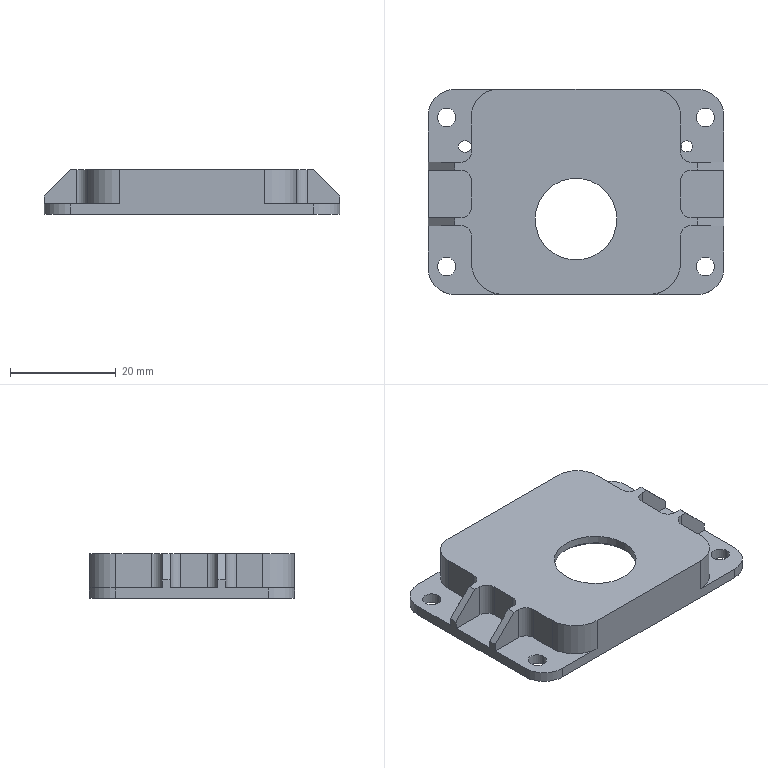Part | 1 solid | 142 faces | box 56 x 38.85 x 8.5 mm | volume 6332 mm3 | plane 80 | cylinder 52 | cone 10 | commonest cylinder face diameters 4 x26 3.5 x8 10 x6 2.1 x4 6 x4 12 x2